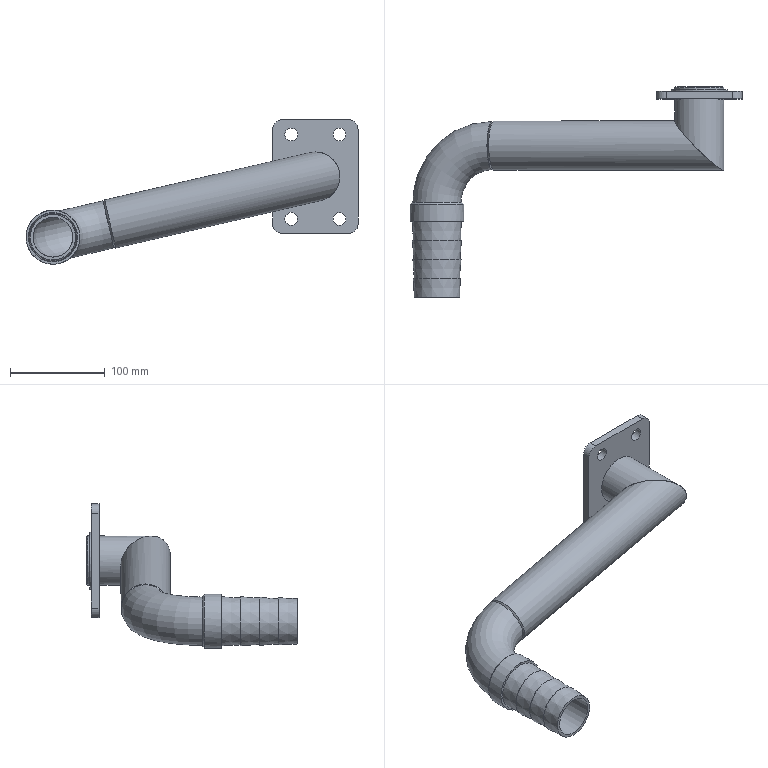Part | STEP file | HL4GZ-1.581.027 (variable pump inlet fitting) | 5 solids | 48 faces | box 350.221 x 222 x 152.386 mm | volume 345083 mm3 | plane 20 | cylinder 17 | cone 9 | torus 2 | commonest cylinder face diameters 13.5 x4 20 x4 52 x3 44 x2 42 x1 57 x1